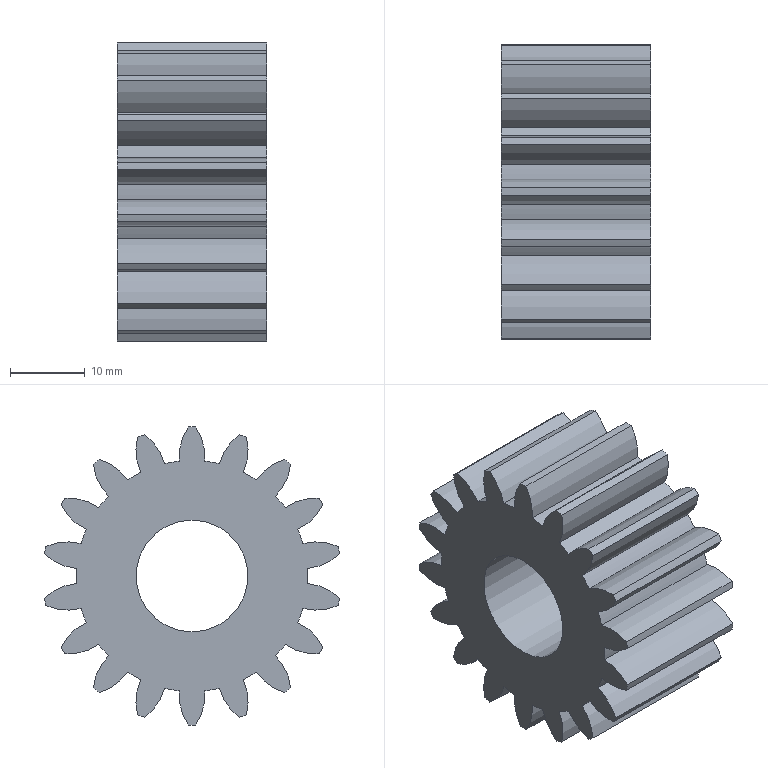Part | STEP file | spur gear_gb_GB - Spur gear 2M 18T 20PA 20FW ---S18A75H50L15.0N | 1 solid | 75 faces | box 20 x 39.557 x 40 mm | volume 16040 mm3 | cylinder 73 | plane 2 | commonest cylinder face diameters 14.4 x36 30.998 x18 40 x18 15 x1